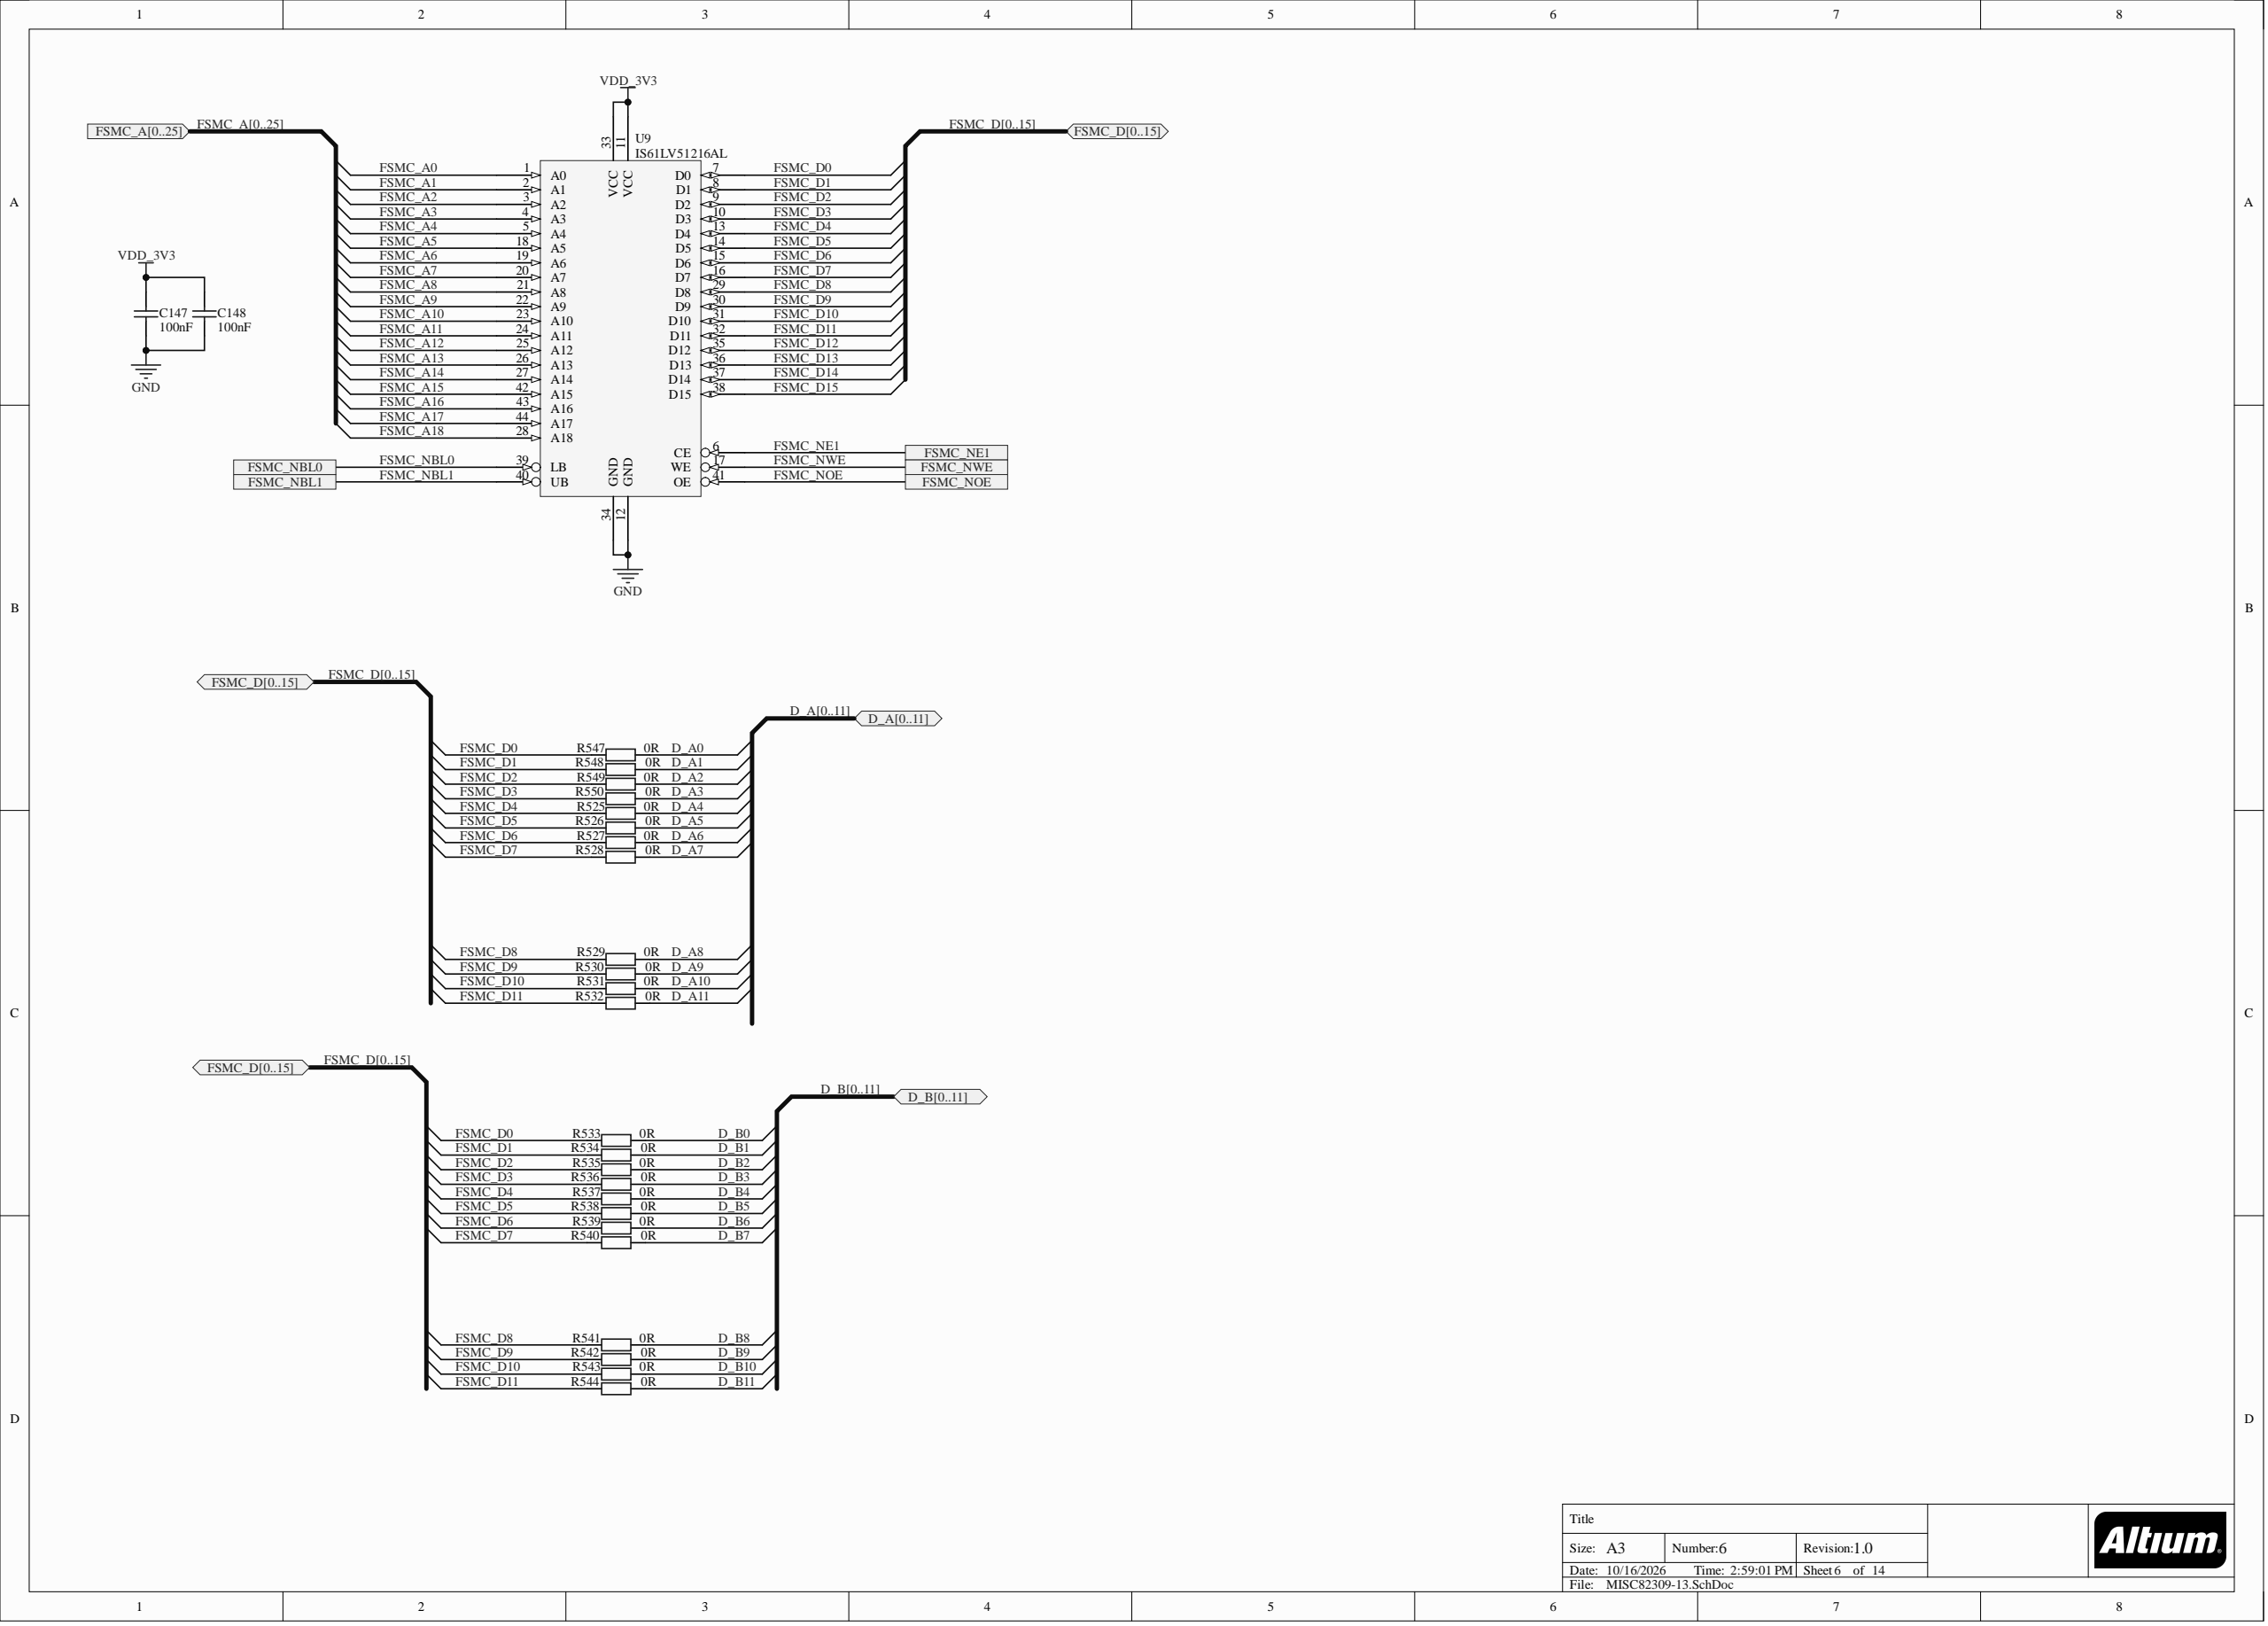Circuit board | Altium Designer | 747 parts | 576 nets | one sheet of the schematic
Parts on this sheet (reference | value | footprint):
C147 | 100nF | C0603
C148 | 100nF | C0603
R525 | 0R | RES_0603
R526 | 0R | RES_0603
R527 | 0R | RES_0603
R528 | 0R | RES_0603
R529 | 0R | RES_0603
R530 | 0R | RES_0603
R531 | 0R | RES_0603
R532 | 0R | RES_0603
R533 | 0R | RES_0603
R534 | 0R | RES_0603
R535 | 0R | RES_0603
R536 | 0R | RES_0603
R537 | 0R | RES_0603
R538 | 0R | RES_0603
R539 | 0R | RES_0603
R540 | 0R | RES_0603
R541 | 0R | RES_0603
R542 | 0R | RES_0603
R543 | 0R | RES_0603
R544 | 0R | RES_0603
R547 | 0R | RES_0603
R548 | 0R | RES_0603
R549 | 0R | RES_0603
R550 | 0R | RES_0603
U9 | IS61LV51216AL | TSOP44-IS61LV51216AL-10TLI
Nets of these parts (net: part-pin ...):
VDD_3V3: C147-2 C148-2 U9-11 U9-33
GND: C147-1 C148-1 U9-12 U9-34
FSMC_NWE: U9-17
FSMC_NOE: U9-41
FSMC_NE1: U9-6
FSMC_NBL1: U9-40
FSMC_NBL0: U9-39
FSMC_D15: U9-38
FSMC_D14: U9-37
FSMC_D13: U9-36
FSMC_D12: U9-35
FSMC_D11: R532-2 R544-2 U9-32
FSMC_D10: R531-2 R543-2 U9-31
FSMC_D9: R530-2 R542-2 U9-30
FSMC_D8: R529-2 R541-2 U9-29
FSMC_D7: R528-2 R540-2 U9-16
FSMC_D6: R527-2 R539-2 U9-15
FSMC_D5: R526-2 R538-2 U9-14
FSMC_D4: R525-2 R537-2 U9-13
FSMC_D3: R536-2 R550-2 U9-10
FSMC_D2: R535-2 R549-2 U9-9
FSMC_D1: R534-2 R548-2 U9-8
FSMC_D0: R533-2 R547-2 U9-7
FSMC_A18: U9-28
FSMC_A17: U9-44
FSMC_A16: U9-43
FSMC_A15: U9-42
FSMC_A14: U9-27
FSMC_A13: U9-26
FSMC_A12: U9-25
FSMC_A11: U9-24
FSMC_A10: U9-23
FSMC_A9: U9-22
FSMC_A8: U9-21
FSMC_A7: U9-20
FSMC_A6: U9-19
FSMC_A5: U9-18
FSMC_A4: U9-5
FSMC_A3: U9-4
FSMC_A2: U9-3
FSMC_A1: U9-2
FSMC_A0: U9-1
D_B11: R544-1
D_B10: R543-1
D_B9: R542-1
D_B8: R541-1
D_B7: R540-1
D_B6: R539-1
D_B5: R538-1
D_B4: R537-1
D_B3: R536-1
D_B2: R535-1
D_B1: R534-1
D_B0: R533-1
D_A11: R532-1
D_A10: R531-1
D_A9: R530-1
D_A8: R529-1
D_A7: R528-1
D_A6: R527-1
D_A5: R526-1
D_A4: R525-1
D_A3: R550-1
D_A2: R549-1
D_A1: R548-1
D_A0: R547-1